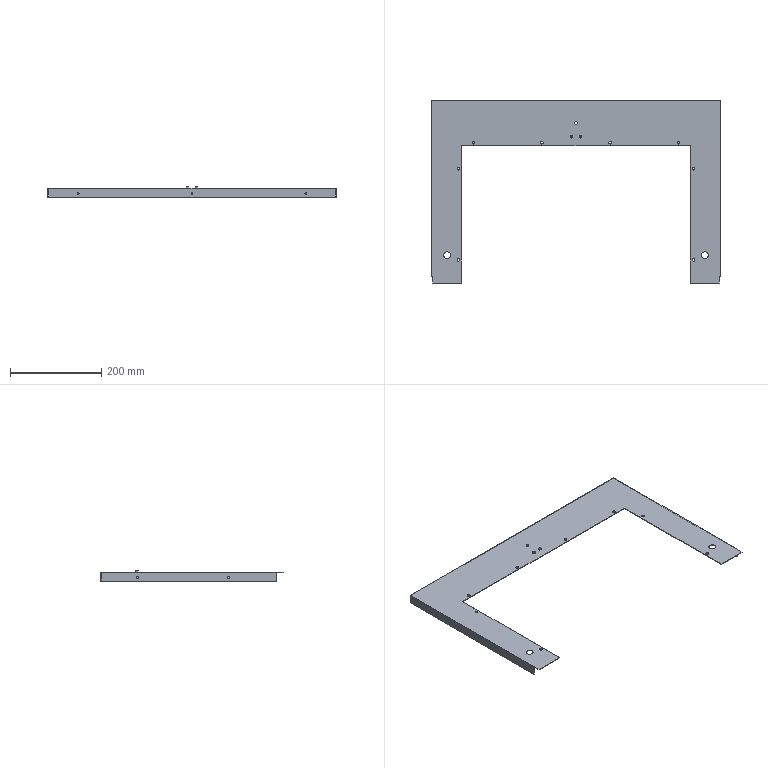Part | STEP file | 3 solids | 82 faces | box 632 x 399.5 x 22.5 mm | volume 152413 mm3 | cylinder 44 | plane 34 | cone 4 | commonest cylinder face diameters 6 x18 4.2 x14 3.3 x8 15 x4